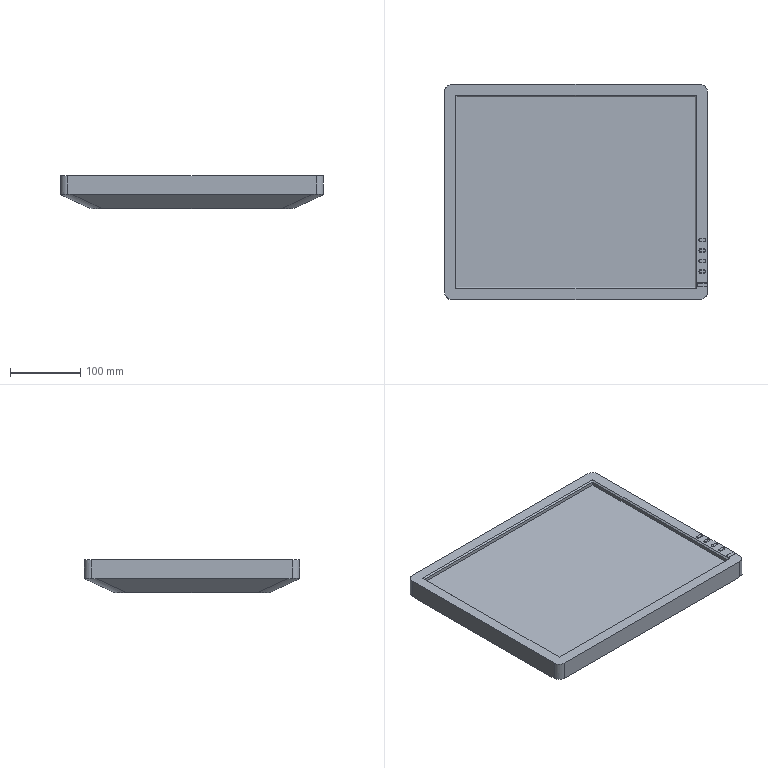Part | SolidWorks | features BaseBody 1, ICE 1 | 1 solid | 99 faces | box 375 x 307 x 47.5 mm | volume 4213214 mm3 | plane 51 | cylinder 40 | cone 8 | commonest cylinder face diameters 5 x20 4 x12 20 x4 80 x4